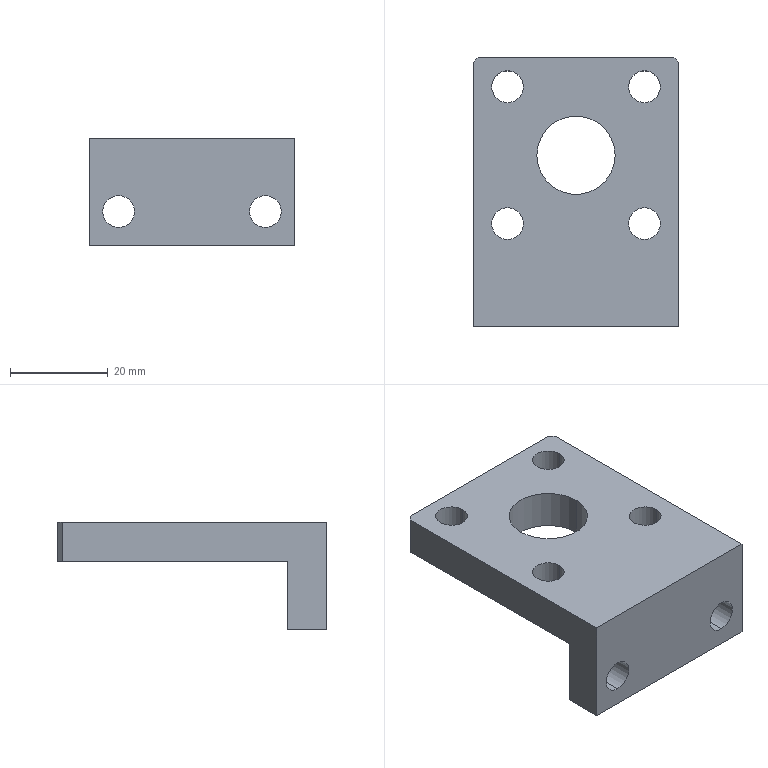Part | STEP file | 001-008-WIB01-25-H35-N5 | 1 solid | 24 faces | box 42 x 55 x 22 mm | volume 19975 mm3 | cylinder 14 | plane 10 | commonest cylinder face diameters 6.5 x12 16 x2